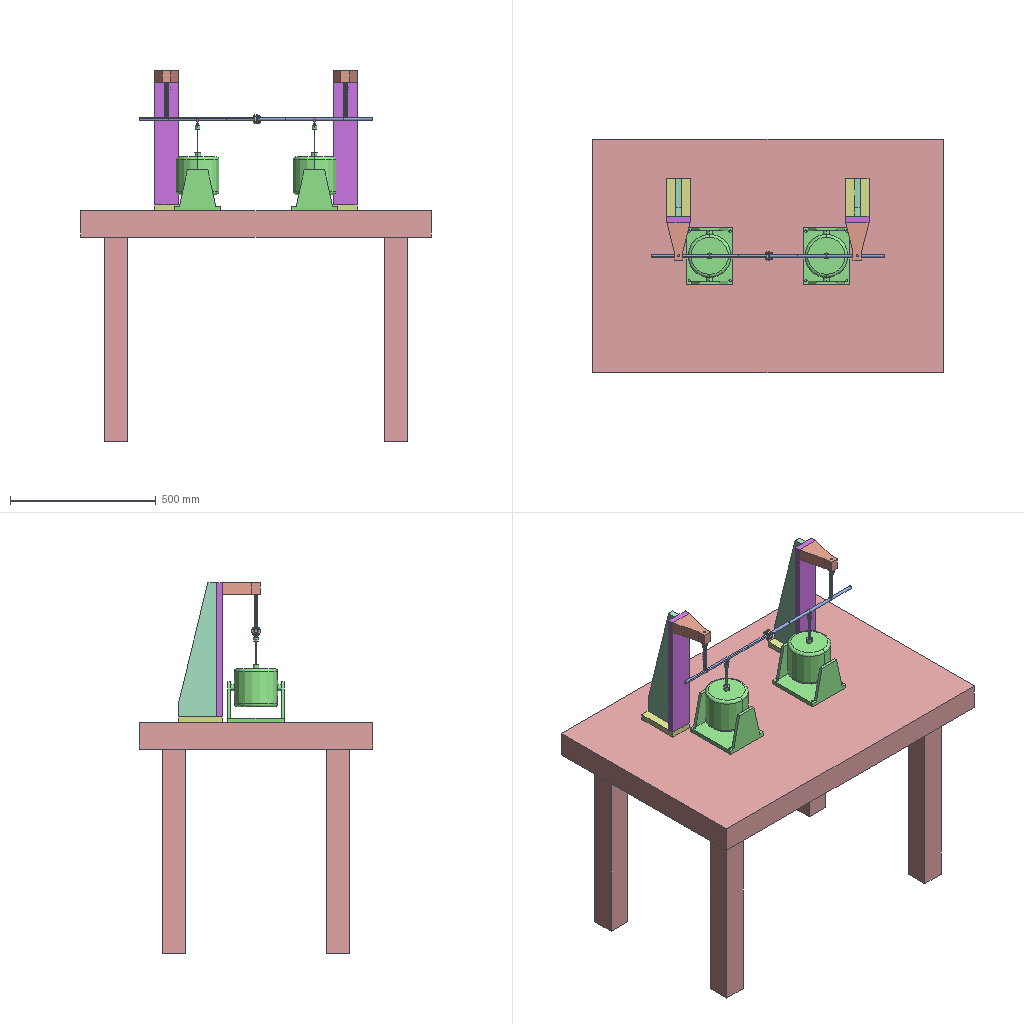Assembly | SolidWorks | 22 different items | 47 placed | box 1200 x 800 x 1270 mm
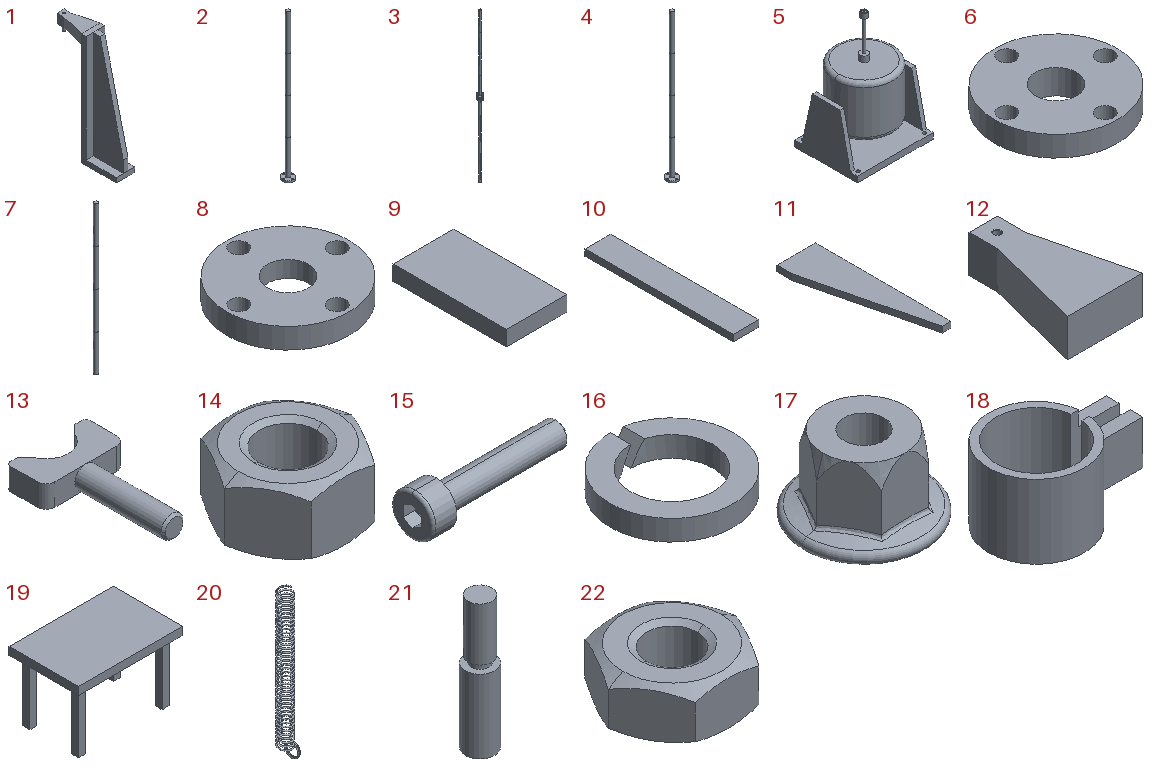Parts list (item | name | quantity | parent item | size | volume | features):
1 | (subassembly) | x2 | - | 80 x 280 x 480 mm | 2019468 mm3 | -
2 | (subassembly) | x1 | in 3 | 30 x 30 x 401 mm | 34403 mm3 | -
3 | (subassembly) | x1 | - | 31.918 x 31.776 x 800 mm | 71021 mm3 | -
4 | (subassembly) | x1 | in 3 | 30 x 30 x 400 mm | 34158 mm3 | -
5 | - | x2 | - | 194.286 x 160 x 295 mm | 2941596 mm3 | features ICE 7, Chamfer 1, Extrusion 1, Fillet 1, HoleWzd 1, MirrorPattern 1
6 | - | x1 | in 2 | 30 x 30 x 6 mm | 2987 mm3 | features ICE 3, Chamfer 1, CirPattern 1, Extrusion 1
7 | - | x2 | in 2, 4 | 10 x 10 x 400 mm | 31416 mm3 | features Extrusion 1, PLine 1
8 | - | x1 | in 4 | 30 x 30 x 5 mm | 2742 mm3 | features ICE 3, Chamfer 1, CirPattern 1, Extrusion 1
9 | - | x2 | in 1 | 80 x 150 x 20 mm | 240000 mm3 | features Extrusion 1
10 | - | x2 | in 1 | 80 x 460 x 20 mm | 736000 mm3 | features Extrusion 1
11 | - | x2 | in 1 | 130 x 460 x 20 mm | 786000 mm3 | features Cut 1, Extrusion 1
12 | - | x2 | in 1 | 80 x 130 x 40 mm | 254543 mm3 | features Extrusion 1, HoleWzd 1
13 | - | x2 | - | 18 x 29 x 5 mm | 980.993 mm3 | features Chamfer 2, Fillet 2, ICE 2, Extrusion 1
14 | - | x2 | - | 9.238 x 8 x 4.7 mm | 190.603 mm3 | features RevCut 2, Chamfer 1, Extrusion 1, LPattern 1
15 | - | x4 | in 3 | 24 x 7 x 7 mm | 386.251 mm3 | features Fillet 2, RevCut 2, Boss 1, Chamfer 1, Cut 1, Extrusion 1, LPattern 1
16 | - | x4 | in 3 | 6.6 x 6.6 x 1.1 mm | 20.135 mm3 | features Cut 1, Extrusion 1
17 | - | x1 | in 3 | 10.5 x 10.5 x 6.5 mm | 259.355 mm3 | features RevCut 2, Chamfer 1, Cut 1, Extrusion 1, Fillet 1, LPattern 1, Revolution 1
18 | - | x2 | - | 18.5 x 13 x 10 mm | 482.242 mm3 | features ICE 2, ExtruThin 1
19 | - | x1 | - | 1200 x 800 x 790 mm | 104320000 mm3 | features MirrorPattern 2, Extrusion 1, ICE 1
20 | - | x2 | - | 14.02 x 12 x 131.993 mm | 1022 mm3 | features Helix 2, RefAxis 2, CompositeCurve 1, ICE 1, Sweep 1
21 | - | x2 | in 1 | 10 x 10 x 45 mm | 2925 mm3 | features ICE 2, Extrusion 1
22 | - | x8 | in 3 | 8.083 x 7 x 3.2 mm | 104.299 mm3 | features RevCut 2, Chamfer 1, Extrusion 1, LPattern 1
Mates (type | each side: item.copy, entity, surface, feature):
In the top assembly
Coincident | 19.1 face plane Boss-Extrude1 | 5.1 face plane Boss-Extrude3
Coincident | 19.1 face plane Boss-Extrude1 | 5.2 face plane Boss-Extrude3
Coincident | 5.1 face plane Boss-Extrude3 | 5.2 face plane Boss-Extrude3
DistanceDim | 5.1 plane | 5.2 plane
Symmetric | 5.1 plane | 5.2 plane | assembly plane
Coincident | 5.1 plane | assembly plane
Concentric | 5.1 face cylinder M5 Tapped Hole1 | 13.1 face cylinder Boss-Extrude2
Concentric | 13.1 face cylinder Boss-Extrude2 | 14.1 face cylinder BaseNut
Coincident | 5.1 face plane Boss-Extrude8 | 14.1 face plane BaseNut
Parallel | 5.1 face plane Boss-Extrude3 | 13.1 face plane Boss-Extrude1
DistanceDim | 13.1 face plane Boss-Extrude1 | 14.1 face plane BaseNut
Concentric | 5.2 face cylinder M5 Tapped Hole1 | 13.2 face cylinder Boss-Extrude2
Parallel | 13.1 face plane Boss-Extrude1 | 13.2 face plane Boss-Extrude1
Coincident | 13.1 face plane Boss-Extrude1 | 13.2 face plane Boss-Extrude1
Concentric | 13.2 face cylinder Boss-Extrude2 | 14.2 face cylinder BaseNut
Coincident | 5.2 face plane Boss-Extrude8 | 14.2 face plane BaseNut
Concentric | 7.1 face cylinder Split Line1 | 13.2 face cylinder Boss-Extrude1
Coincident | 19.1 face plane Boss-Extrude1 | 9.1 face plane Boss-Extrude1
Coincident | 19.1 face plane Boss-Extrude1 | 9.2 face plane Boss-Extrude1
Coincident | 10.1 face plane Boss-Extrude1 | 10.2 face plane Boss-Extrude1
Concentric | 21.1 face cylinder Boss-Extrude1 | 20.1 axis
Perpendicular | 1.1 plane | 20.1 axis
Concentric | 21.2 face cylinder Boss-Extrude1 | 20.2 axis
Coincident | 20.1 axis | 20.2 axis
Concentric | 7.2 face cylinder Split Line1 | 20.1 axis
Coincident | 8.1 face plane Boss-Extrude1 | assembly plane
Concentric | 21.1 face cylinder Boss-Extrude1 | 18.1 face cylinder Extrude-Thin1
Coincident | 21.1 face plane Boss-Extrude1 | 18.1 face plane Extrude-Thin1
Concentric | 21.2 face cylinder Boss-Extrude1 | 18.2 face cylinder Extrude-Thin1
Coincident | 21.2 face plane Boss-Extrude1 | 18.2 face plane Extrude-Thin1
In subassembly 1
Coincident | 9.3 face plane Boss-Extrude1 | 10.3 face plane Boss-Extrude1 | 3 times
Coincident | 10.3 face plane Boss-Extrude1 | 11.1 face plane Boss-Extrude1
Coincident | 9.3 face plane Boss-Extrude1 | 11.1 face plane Boss-Extrude1
Coincident | 10.3 face plane Boss-Extrude1 | 12.1 face plane Boss-Extrude1
Coincident | 10.3 face plane Boss-Extrude1 | 12.1 edge | 2 times
Concentric | 12.1 face cylinder M8 Tapped Hole1 | 21.3 face cylinder Boss-Extrude2
Coincident | 12.1 face plane Boss-Extrude1 | 21.3 face plane Boss-Extrude1
Coincident | 11.1 plane | 1.2 plane
In subassembly 3
Concentric | 8.2 face cylinder Cut-Extrude2 | 6.1 face cylinder Boss-Extrude2
Coincident | 8.2 face plane Boss-Extrude1 | 6.1 face plane Boss-Extrude1
Concentric | 8.2 face cylinder CirPattern1 | 6.1 face cylinder CirPattern1
Concentric | 15.1 face cylinder BaseBody | 16.1 face cylinder Base-Extrude
Coincident | 15.1 face plane BaseHead | 16.1 face plane Base-Extrude
Concentric | 8.2 face cylinder CirPattern1 | 15.1 face cylinder BaseBody
Coincident | 8.2 face plane Boss-Extrude1 | 16.1 face plane Base-Extrude
Concentric | 15.1 face cylinder BaseBody | 17.1 face
Coincident | 6.1 face plane Boss-Extrude1 | 17.1 face
Concentric | 15.1 face cylinder BaseBody | 22.1 face cylinder BaseNut
Coincident | 6.1 face plane Boss-Extrude1 | 22.1 face plane BaseNut
Concentric | 15.1 face cylinder BaseBody | 22.2 face cylinder BaseNut
Coincident | 22.1 face plane BaseNut | 22.2 face plane BaseNut
Concentric | 15.2 face cylinder BaseBody | 16.2 face cylinder Base-Extrude
Coincident | 15.2 face plane BaseHead | 16.2 face plane Base-Extrude
Concentric | 15.2 face cylinder BaseBody | 22.3 face cylinder BaseNut
Concentric | 15.2 face cylinder BaseBody | 22.4 face cylinder BaseNut
Coincident | 22.3 face plane BaseNut | 22.4 face plane BaseNut
Coincident | 8.2 face plane Boss-Extrude1 | 16.2 face plane Base-Extrude
Coincident | 6.1 face plane Boss-Extrude1 | 22.3 face plane BaseNut
Concentric | 8.2 face cylinder Cut-Extrude1 | 15.2 face cylinder BaseBody
Concentric | 6.1 face cylinder CirPattern1 | 15.2 face cylinder BaseBody
Concentric | 15.3 face cylinder BaseBody | 16.3 face cylinder Base-Extrude
Coincident | 15.3 face plane BaseHead | 16.3 face plane Base-Extrude
Concentric | 15.3 face cylinder BaseBody | 22.5 face cylinder BaseNut
Concentric | 15.3 face cylinder BaseBody | 22.6 face cylinder BaseNut
Coincident | 22.5 face plane BaseNut | 22.6 face plane BaseNut
Coincident | 8.2 face plane Boss-Extrude1 | 16.3 face plane Base-Extrude
Coincident | 6.1 face plane Boss-Extrude1 | 22.5 face plane BaseNut
Concentric | 8.2 face cylinder CirPattern1 | 15.3 face cylinder BaseBody
Concentric | 6.1 face cylinder Cut-Extrude1 | 15.3 face cylinder BaseBody
Concentric | 15.4 face cylinder BaseBody | 16.4 face cylinder Base-Extrude
Coincident | 15.4 face plane BaseHead | 16.4 face plane Base-Extrude
Concentric | 15.4 face cylinder BaseBody | 22.7 face cylinder BaseNut
Concentric | 15.4 face cylinder BaseBody | 22.8 face cylinder BaseNut
Coincident | 22.7 face plane BaseNut | 22.8 face plane BaseNut
Coincident | 8.2 face plane Boss-Extrude1 | 16.4 face plane Base-Extrude
Coincident | 6.1 face plane Boss-Extrude1 | 22.7 face plane BaseNut
Concentric | 8.2 face cylinder CirPattern1 | 15.4 face cylinder BaseBody
Concentric | 6.1 face cylinder CirPattern1 | 15.4 face cylinder BaseBody
In subassembly 2
Concentric | 7.3 face cylinder Split Line1 | 6.2 face cylinder Cut-Extrude3
Coincident | 7.3 face plane Boss-Extrude1 | 6.2 face plane Boss-Extrude1
Coincident | 7.3 plane | 6.2 plane
In subassembly 4
Concentric | 7.3 face cylinder Split Line1 | 8.3 face cylinder Cut-Extrude3
Coincident | 7.3 face plane Boss-Extrude1 | 8.3 face plane Boss-Extrude1
Coincident | 7.3 plane | 8.3 plane